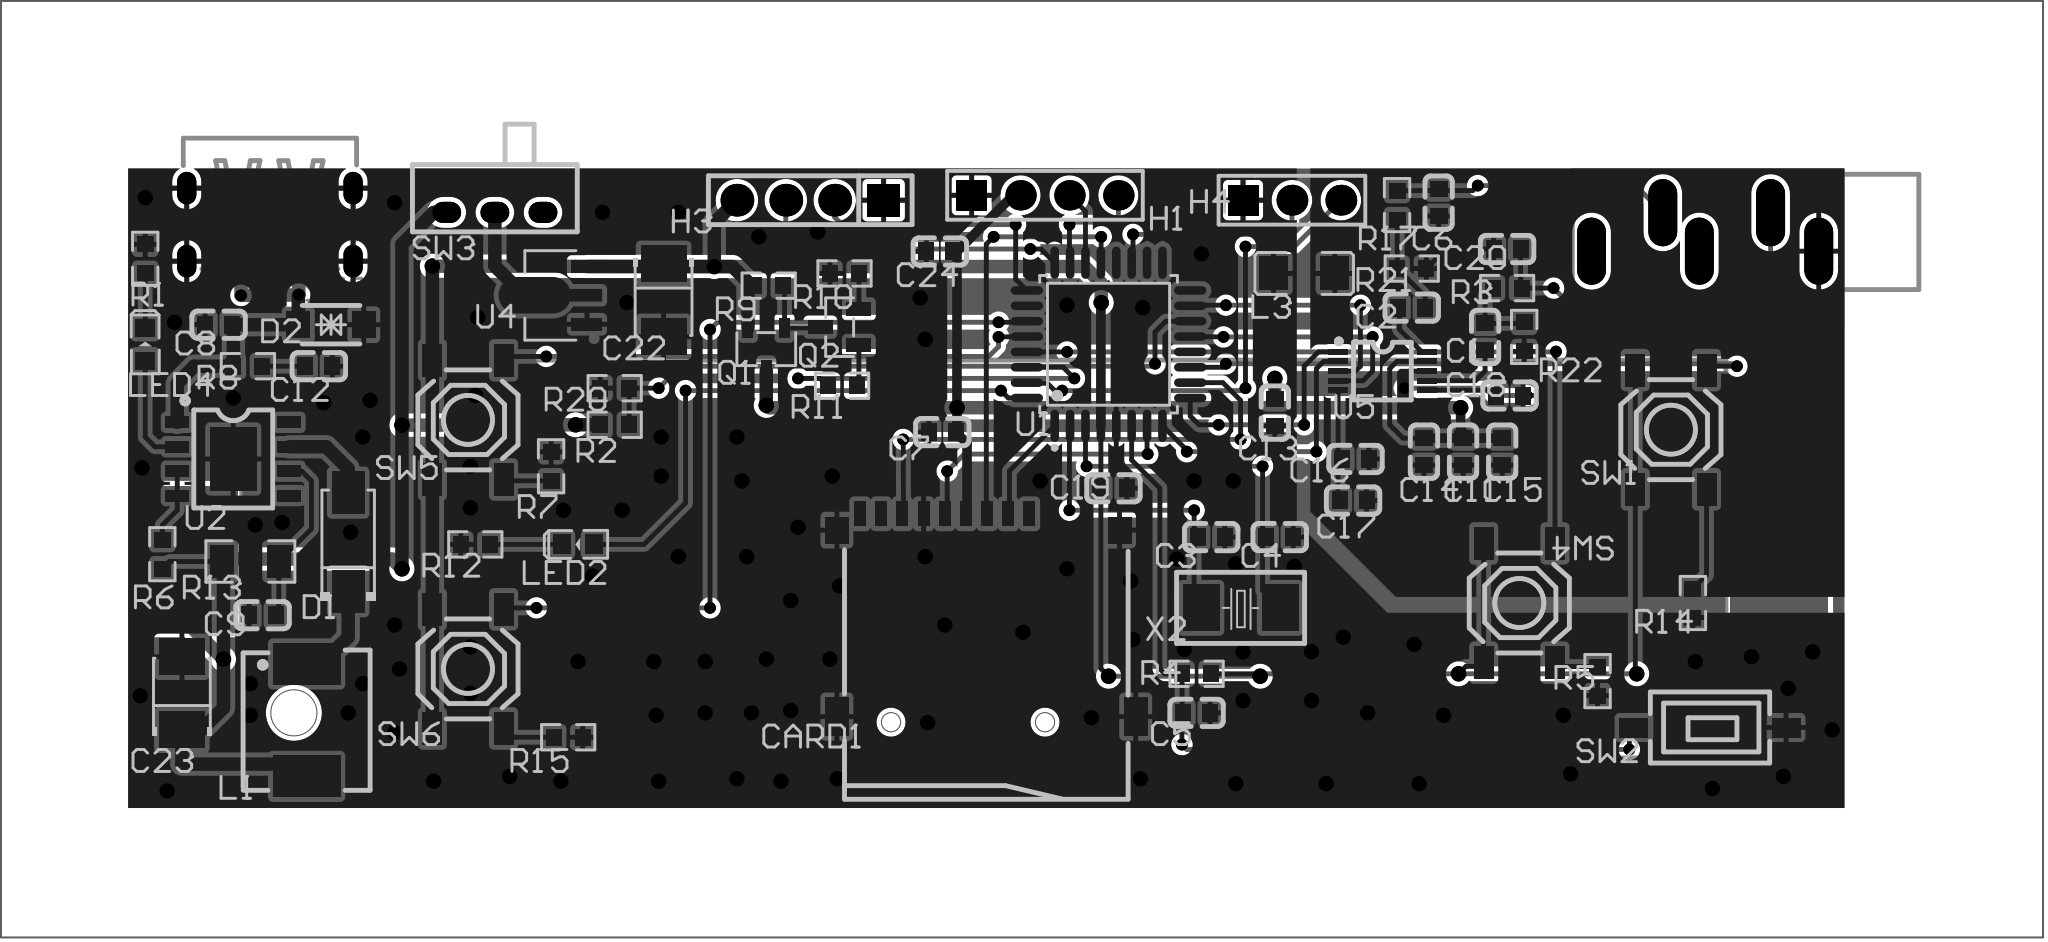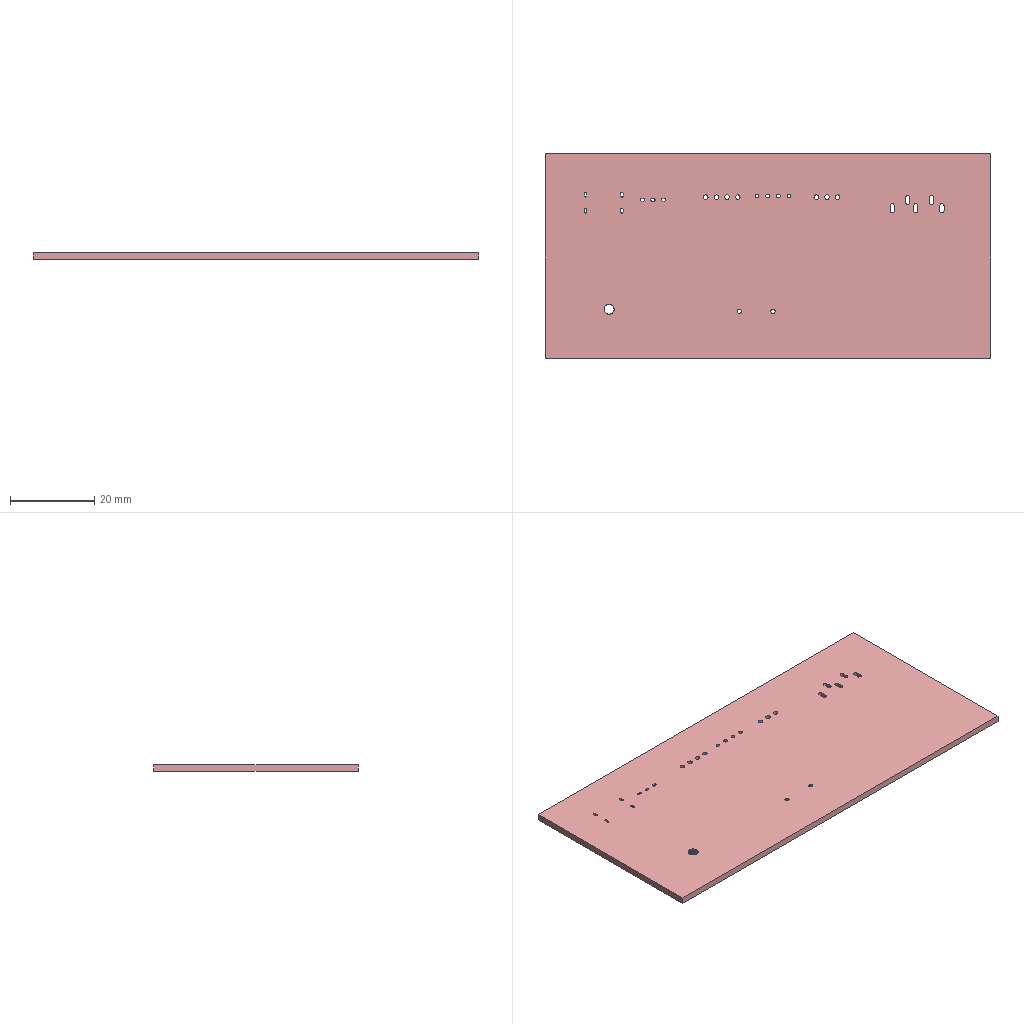Circuit board layout | Altium Designer | box 106.1 x 48.7 x 1.6 mm
Layer stack:
# Altium Designer layer stack of  (unit mm; dielectric type: 0 none, 1 core, 2 prepreg, 3 surface material)
index,name,kind,layer,copper_thickness_mm,dielectric_type,dielectric_thickness_mm,dielectric_material,dielectric_constant
0,Top Paste Mask Layer,other,,,,,,
1,Top Silkscreen Layer,other,,,,,,
2,Top Solder Mask Layer,dielectric,,,3,0.0102,,3.3
3,Top Layer,copper,Top Layer,0.0356,,,,
4,Dielectric1,dielectric,,,3,1.509,FR4,4.5
5,Bottom Layer,copper,Bottom Layer,0.0356,,,,
6,Bottom Solder Mask Layer,dielectric,,,3,0.0102,,3.3
7,Bottom Silkscreen Layer,other,,,,,,
8,Bottom Paste Mask Layer,other,,,,,,
# drill layer pairs: low layer,high layer
drill_pair,Top Layer,Bottom Layer
Part placement:
Designator,Comment,Layer,Footprint,Center-X(mm),Center-Y(mm),Rotation
J1,PJ-325M/3.5MM,BottomLayer,AUDIO-TH_PJ-325C,158.369,106.553,180
BT1,BH-18650-B1BA002,BottomLayer,BATTERY-SMD_18650-1S-L77.1-W20.7-1,120.904,89.535,270
C8,22uf,TopLayer,C0603,81.153,101.727,0
C9,22uF,TopLayer,C0603,83.439,86.614,0
C12,10uF,TopLayer,C0603,86.36,99.568,180
C24,0.1uf,TopLayer,C0603,118.618,105.537,0
C7,0.1uf,TopLayer,C0603,118.745,96.139,0
C19,2.2uf,TopLayer,C0603,127.635,93.218,180
C5,10u,TopLayer,C0603,131.953,81.534,180
C3,20p,TopLayer,C0603,132.715,90.678,180
C4,20p,TopLayer,C0603,136.271,90.678,180
C13,10u,TopLayer,C0603,136.017,97.155,90
C17,10u,TopLayer,C0603,140.081,92.583,180
C16,0.1u,TopLayer,C0603,140.208,94.742,180
C2,2.2uF,TopLayer,C0603,143.129,102.616,0
C14,2.2uf,TopLayer,C0603,143.764,95.123,90
C6,2.2nf,TopLayer,C0603,144.526,108.077,90
C11,0.1u,TopLayer,C0603,145.796,95.123,90
C1,2.2uF,TopLayer,C0603,146.939,101.092,90
C20,2.2nf,TopLayer,C0603,148.082,105.664,180
C18,10u,TopLayer,C0603,148.209,98.044,180
C15,10nf,TopLayer,C0603,147.828,95.123,90
C23,22uF,TopLayer,CAP-SMD_L3.5-W2.8-R-RD,79.248,82.551,270
C22,22uF,TopLayer,CAP-SMD_L3.5-W2.8-R-RD,104.267,102.998,90
X2,8MHz,TopLayer,CRYSTAL-SMD_L5.0-W3.2,134.239,86.995,0
U2,IP5306,TopLayer,ESOP-8_L4.9-W3.9-P1.27-LS6.0-BL-EP,81.915,94.742,270
H1,HDR-F-2.54_1x4,TopLayer,HDR-F-2.54_1X4,124.079,108.458,0
H4,Z-211-0311-0021-001,TopLayer,HDR-TH_3P-P2.54-V-M-1,136.906,108.204,0
H3,220S-1*4P H=8.5MM,TopLayer,HDR-TH_4P-P2.54-V-F,111.887,108.204,180
L1,1uH,TopLayer,IND-SMD_L6.8-W6.8_SMMS0630,85.725,81.153,270
L3,600Ω,TopLayer,L1206,137.541,104.394,180
LED4,LED-0603_G,TopLayer,LED0603_GREEN,77.343,100.711,90
LED2,LED-0603_G,TopLayer,LED0603_GREEN,99.822,90.297,180
U1,STM32G070KBT6,TopLayer,LQFP-32_L7.0-W7.0-P0.80-LS9.0-BL,127.381,100.711,0
R1,10k,TopLayer,R0603,77.343,105.156,90
R6,120,TopLayer,R0603,78.232,89.789,270
R8,120,TopLayer,R0603,82.677,99.568,0
R12,10k,TopLayer,R0603,94.488,90.297,0
R7,10K,TopLayer,R0603,98.425,94.361,270
R15,10K,TopLayer,R0603,99.314,80.264,180
R20,100k,TopLayer,R0603,101.727,98.425,0
R2,47k,TopLayer,R0603,101.727,96.52,180
R9,1M,TopLayer,R0603,109.728,103.759,0
R11,10K,TopLayer,R0603,113.538,98.552,0
R10,100K,TopLayer,R0603,113.665,104.394,180
R4,1k,TopLayer,R0603,131.953,83.566,0
R17,470R,TopLayer,R0603,142.367,107.95,270
R21,NA,TopLayer,R0603,143.129,104.648,0
R3,470R,TopLayer,R0603,148.082,103.632,180
R22,NA,TopLayer,R0603,148.971,101.092,90
R5,10K,TopLayer,R0603,152.781,83.185,90
R14,10K,TopLayer,R0603,157.734,87.249,90
R13,0R5,TopLayer,R1206,82.804,89.408,180
D1,SS14,TopLayer,SMA_L4.2-W2.6-LS5.3-RD,87.884,90.424,90
D2,SMF6.0CA,TopLayer,SOD-123FL_L2.8-W1.8-LS3.7-BI,86.995,101.727,180
Q2,SI2302_C351401,TopLayer,SOT-23-3_L2.9-W1.3-P1.90-LS2.4,113.412,101.597,0
Q1,SI2301CDS-T1-GE3,TopLayer,SOT-23-3_L3.0-W1.7-P0.95-LS2.9-BR,109.601,100.457,90
U4,HT7833,TopLayer,SOT-89_L4.5-W2.5-P1.50-LS4.2-BR,99.129,103.251,0
SW5,TS-1187A-B-A-B,TopLayer,SW-SMD_4P-L5.1-W5.1-P3.70-LS6.5-TL-2,94.107,96.774,90
SW6,TS-1187A-B-A-B,TopLayer,SW-SMD_4P-L5.1-W5.1-P3.70-LS6.5-TL-2,94.107,83.82,90
SW4,TS-1187A-B-A-B,TopLayer,SW-SMD_4P-L5.1-W5.1-P3.70-LS6.5-TL-2,148.717,87.249,90
SW1,TS-1187A-B-A-B,TopLayer,SW-SMD_4P-L5.1-W5.1-P3.70-LS6.5-TL-2,156.591,96.266,90
SW2,TS-1092S-B3D2-G,TopLayer,SW-SMD_L6.1-W3.6-LS7.9,158.623,80.772,180
SW3,MK-12D18-G020,TopLayer,SW-TH_MK-12D18-G040,95.504,107.569,180
CARD1,TF-01A,TopLayer,TF-SMD_TF-01A,121.031,86.614,0
U5,CS4344,TopLayer,TSSOP-10_L3.0-W3.0-P0.50-LS4.9-BL,141.605,99.314,270
USB2,TYPE-C 6P,BottomLayer,TYPE-C-SMD_TYPE-C-6P,83.82,106.807,0
Pad and via stacks:
# Altium Designer via and pad stacks of  (unit mm). Each distinct definition once, with the count of objects using it.
# via: kind,start_layer,end_layer,hole_mm,diameter_mm,mode(0 simple;1 top-mid-bottom;2 full stack),diameter_per_layer,count,example_net
# pad: kind,layer,hole_mm,hole_type(0 round;1 square;2 slot),plating,top_size,top_shape(1 round;2 rect;3 octagon;9 rounded rect),mid_size,bottom_size,mode,footprint,size_per_layer,count,example
pad,Multi-Layer,1.001,2,plated,1.501x3.5,1,1.501x3.5,1.501x3.5,0,AUDIO-TH_PJ-325C,,5,J1.5
pad,Multi-Layer,0.889,0,plated,1.575x1.575,2,1.575x1.575,1.575x1.575,0,HDR-F-2.54_1X4,,1,H1.1
pad,Multi-Layer,0.889,0,plated,1.575x1.575,1,1.575x1.575,1.575x1.575,0,HDR-F-2.54_1X4,,3,H1.2
pad,Multi-Layer,1.1,0,plated,1.6x1.6,1,1.6x1.6,1.6x1.6,0,HDR-TH_3P-P2.54-V-M-1,,2,H4.3
pad,Multi-Layer,1.1,0,plated,1.575x1.6,2,1.575x1.6,1.575x1.6,0,HDR-TH_3P-P2.54-V-M-1,,1,H4.1
pad,Multi-Layer,1.1,0,plated,1.699x1.699,2,1.699x1.699,1.699x1.699,0,HDR-TH_4P-P2.54-V-F,,1,H3.1
pad,Multi-Layer,1.1,0,plated,1.699x1.699,1,1.699x1.699,1.699x1.699,0,HDR-TH_4P-P2.54-V-F,,3,H3.2
pad,Multi-Layer,0.5994,2,plated,1.1x1.501,1,1.1x1.501,1.1x1.501,0,SW-TH_MK-12D18-G040,,3,SW3.1
pad,Multi-Layer,0.5004,2,plated,1.001x1.699,1,1.001x1.699,1.001x1.699,0,TYPE-C-SMD_TYPE-C-6P,,4,USB2.7
pad,Bottom Layer,0,0,plated,7.62x5.08,2,7.62x5.08,7.62x5.08,0,BATTERY-SMD_18650-1S-L77.1-W20.7-1,,2,BT1.1
pad,Bottom Layer,0,0,plated,0.8001x1.199,2,0.8001x1.199,0.8001x1.199,0,TYPE-C-SMD_TYPE-C-6P,,2,USB2.B12
pad,Bottom Layer,0,0,plated,0.701x1.199,2,0.701x1.199,0.701x1.199,0,TYPE-C-SMD_TYPE-C-6P,,4,USB2.B9
pad,Top Layer,0,0,plated,0.8001x0.8992,2,0.8001x0.8992,0.8001x0.8992,0,C0603,,40,C8.2
pad,Top Layer,0,0,plated,1.9x2.375,2,1.9x2.375,1.9x2.375,0,CAP-SMD_L3.5-W2.8-R-RD,,4,C23.1
pad,Top Layer,0,0,plated,1.9x2.4,2,1.9x2.4,1.9x2.4,0,CRYSTAL-SMD_L5.0-W3.2,,2,X2.2
pad,Top Layer,0,0,plated,0.5994x1.199,2,0.5994x1.199,0.5994x1.199,0,ESOP-8_L4.9-W3.9-P1.27-LS6.0-BL-EP,,8,U2.1
pad,Top Layer,0,0,plated,3.3x2.4,2,3.3x2.4,3.3x2.4,0,ESOP-8_L4.9-W3.9-P1.27-LS6.0-BL-EP,,1,U2.9
pad,Top Layer,0,0,plated,2.149x3.5,2,2.149x3.5,2.149x3.5,0,IND-SMD_L6.8-W6.8_SMMS0630,,2,L1.2
pad,Top Layer,0,0,plated,1.486x1.727,2,1.486x1.727,1.486x1.727,0,L1206,,2,L3.2
pad,Top Layer,0,0,plated,1.001x0.8992,2,1.001x0.8992,1.001x0.8992,0,LED0603_GREEN,,4,LED4.2
pad,Top Layer,0,0,plated,0.447x1.684,1,0.447x1.684,0.447x1.684,0,LQFP-32_L7.0-W7.0-P0.80-LS9.0-BL,,16,U1.1
pad,Top Layer,0,0,plated,1.684x0.447,1,1.684x0.447,1.684x0.447,0,LQFP-32_L7.0-W7.0-P0.80-LS9.0-BL,,16,U1.9
pad,Top Layer,0,0,plated,0.8077x0.8636,2,0.8077x0.8636,0.8077x0.8636,0,R0603,,36,R1.2
pad,Top Layer,0,0,plated,1.206x1.702,2,1.206x1.702,1.206x1.702,0,R1206,,2,R13.2
pad,Top Layer,0,0,plated,2.2x1.699,2,2.2x1.699,2.2x1.699,0,SMA_L4.2-W2.6-LS5.3-RD,,2,D1.1
pad,Top Layer,0,0,plated,1.199x1.399,2,1.199x1.399,1.199x1.399,0,SOD-123FL_L2.8-W1.8-LS3.7-BI,,2,D2.1
pad,Top Layer,0,0,plated,1.25x0.701,2,1.25x0.701,1.25x0.701,0,SOT-23-3_L2.9-W1.3-P1.90-LS2.4,,3,Q2.3
pad,Top Layer,0,0,plated,1.036x0.5309,2,1.036x0.5309,1.036x0.5309,0,SOT-23-3_L3.0-W1.7-P0.95-LS2.9-BR,,3,Q1.1
pad,Top Layer,0,0,plated,0.95x0.95,1,0.95x0.95,0.95x0.95,0,SOT-89_L4.5-W2.5-P1.50-LS4.2-BR,,1,U4.2
pad,Top Layer,0,0,plated,1.575x0.6731,2,1.575x0.6731,1.575x0.6731,0,SOT-89_L4.5-W2.5-P1.50-LS4.2-BR,,2,U4.3
pad,Top Layer,0,0,plated,1.699x1.001,2,1.699x1.001,1.699x1.001,0,SW-SMD_4P-L5.1-W5.1-P3.70-LS6.5-TL-2,,16,SW5.1
pad,Top Layer,0,0,plated,1.501x1.001,2,1.501x1.001,1.501x1.001,0,SW-SMD_L6.1-W3.6-LS7.9,,2,SW2.2
pad,Top Layer,0,0,plated,0.5994x1.3,2,0.5994x1.3,0.5994x1.3,0,TF-SMD_TF-01A,,9,CARD1.1
pad,Top Layer,0,0,plated,1.199x1.399,2,1.199x1.399,1.199x1.399,0,TF-SMD_TF-01A,,2,CARD1.10
pad,Top Layer,0,0,plated,1.199x1.999,2,1.199x1.999,1.199x1.999,0,TF-SMD_TF-01A,,2,CARD1.12
pad,Top Layer,0,0,plated,1.001x0.2997,2,1.001x0.2997,1.001x0.2997,0,TSSOP-10_L3.0-W3.0-P0.50-LS4.9-BL,,10,U5.1
via,Top Layer,Bottom Layer,0.3988,0.8001,0,,116,GND
via,Top Layer,Bottom Layer,0.3099,0.6096,0,,47,VCC5.0-USB
via,Top Layer,Bottom Layer,0.3048,0.6096,0,,2,A-GND
Copper pours:
name,layer,net,type(0 solid;1 hatched;2 none)
Top Layer-GND,Top Layer,GND,0
Top Layer-A-GND,Top Layer,A-GND,0
Bottom Layer-GND,Bottom Layer,GND,0
Design rules, without the lines most boards share:
# Altium Designer design rules of  (exported by Altium Designer, unit mm)
# columns: name | kind | enabled | priority | scope1 | scope2 | descriptor | typed fields (field=value)
HoleToHoleClearance | 52 | enabled | 1 | All | All | Hole To Hole Clearance (Gap=10mil) (All),(All) | gap=0.254
copperThickness1oz | 0 | enabled | 1 | All | All | Clearance Constraint (Gap=7mil) (All),(All) | gap=0.1778
copperThickness1oz_1 | 63 | enabled | 1 | All | All | Board Clearance Constraint (Gap=0mil) (All) |
copperThickness2oz | 0 | enabled | 2 | All | All | Clearance Constraint (Gap=7mil) (All),(All) | gap=0.1778
copperThickness2oz_1 | 63 | enabled | 2 | All | All | Board Clearance Constraint (Gap=0mil) (All) |
otherClearance | 0 | enabled | 3 | All | All | Clearance Constraint (Gap=7mil) (All),(All) | gap=0.1778
otherClearance_1 | 63 | enabled | 3 | All | All | Board Clearance Constraint (Gap=0mil) (All) |
copperThickness1oz_2 | 2 | enabled | 1 | All | All | Width Constraint (Min=5mil) (Max=100mil) (Preferred=10mil) (All) |
copperThickness2oz_2 | 2 | enabled | 2 | All | All | Width Constraint (Min=8mil) (Max=100mil) (Preferred=10mil) (All) |
viaSize | 11 | enabled | 1 | All | All | Routing Via (MinHoleWidth=11.811mil) (MaxHoleWidth=248.031mil) (PreferredHoleWidth=12.008mil) (MinWidth=11.811mil) (MaxWidth=248.031mil) (PreferedWidth=12.008mil) (All) | via_min_hole=0.3 via_max_hole=6.3 via_preferred_diameter=0.305 via_preferred_hole=0.305